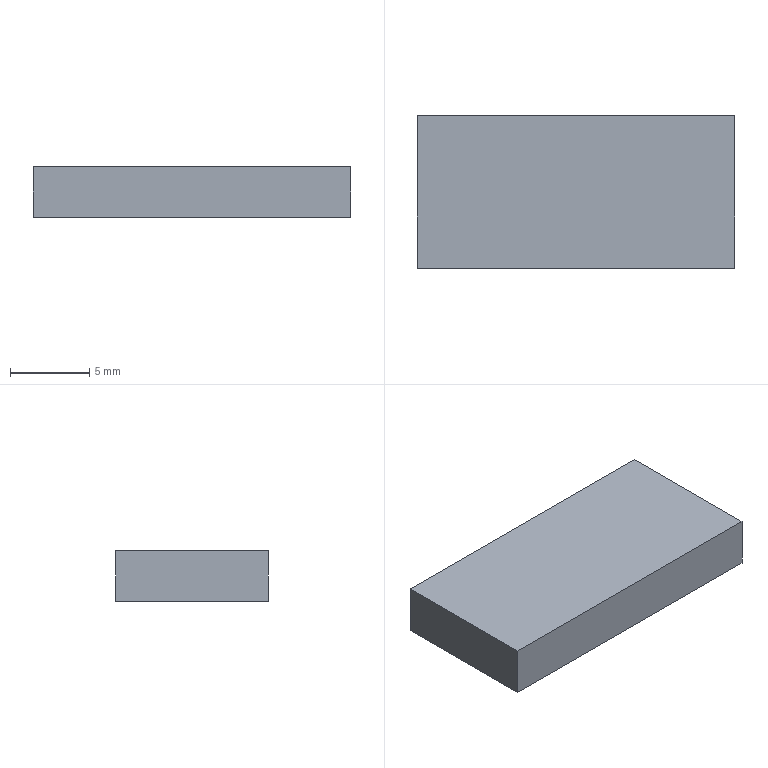Part | SolidWorks | features FlatPattern 1, SMBaseFlange 1, SheetMetal 1 | 1 solid | 6 faces | box 20 x 9.6 x 3.2 mm | volume 614.4 mm3 | plane 6
STEP:
#1=CARTESIAN_POINT('',(25.558,-133.501,0.));
#2=VERTEX_POINT('',#1);
#3=CARTESIAN_POINT('',(25.558,-123.901,0.));
#4=VERTEX_POINT('',#3);
#5=CARTESIAN_POINT('',(25.558,-123.901,0.));
#6=DIRECTION('',(0.,1.,0.));
#7=VECTOR('',#6,1000.);
#8=LINE('',#5,#7);
#9=EDGE_CURVE('',#2,#4,#8,.T.);
#10=ORIENTED_EDGE('',*,*,#9,.F.);
#11=CARTESIAN_POINT('',(25.558,-133.501,-3.2));
#12=VERTEX_POINT('',#11);
#13=CARTESIAN_POINT('',(25.558,-133.501,-3.2));
#14=DIRECTION('',(0.,0.,1.));
#15=VECTOR('',#14,1000.);
#16=LINE('',#13,#15);
#17=EDGE_CURVE('',#12,#2,#16,.T.);
#18=ORIENTED_EDGE('',*,*,#17,.F.);
#19=CARTESIAN_POINT('',(25.558,-123.901,-3.2));
#20=VERTEX_POINT('',#19);
#21=CARTESIAN_POINT('',(25.558,-123.901,-3.2));
#22=DIRECTION('',(0.,1.,0.));
#23=VECTOR('',#22,1000.);
#24=LINE('',#21,#23);
#25=EDGE_CURVE('',#12,#20,#24,.T.);
#26=ORIENTED_EDGE('',*,*,#25,.T.);
#27=CARTESIAN_POINT('',(25.558,-123.901,-3.2));
#28=DIRECTION('',(0.,0.,1.));
#29=VECTOR('',#28,1000.);
#30=LINE('',#27,#29);
#31=EDGE_CURVE('',#20,#4,#30,.T.);
#32=ORIENTED_EDGE('',*,*,#31,.T.);
#33=EDGE_LOOP('',(#10,#18,#26,#32));
#34=FACE_OUTER_BOUND('',#33,.T.);
#35=CARTESIAN_POINT('',(25.558,-123.901,-3.2));
#36=DIRECTION('',(1.,0.,0.));
#37=DIRECTION('',(0.,0.,-1.));
#38=AXIS2_PLACEMENT_3D('',#35,#36,#37);
#39=PLANE('',#38);
#40=ADVANCED_FACE('',(#34),#39,.T.);
#41=CARTESIAN_POINT('',(5.558,-133.501,0.));
#42=VERTEX_POINT('',#41);
#43=CARTESIAN_POINT('',(25.558,-133.501,0.));
#44=DIRECTION('',(1.,0.,0.));
#45=VECTOR('',#44,1000.);
#46=LINE('',#43,#45);
#47=EDGE_CURVE('',#42,#2,#46,.T.);
#48=ORIENTED_EDGE('',*,*,#47,.F.);
#49=CARTESIAN_POINT('',(5.558,-133.501,-3.2));
#50=VERTEX_POINT('',#49);
#51=CARTESIAN_POINT('',(5.558,-133.501,-3.2));
#52=DIRECTION('',(0.,0.,1.));
#53=VECTOR('',#52,1000.);
#54=LINE('',#51,#53);
#55=EDGE_CURVE('',#50,#42,#54,.T.);
#56=ORIENTED_EDGE('',*,*,#55,.F.);
#57=CARTESIAN_POINT('',(25.558,-133.501,-3.2));
#58=DIRECTION('',(1.,0.,0.));
#59=VECTOR('',#58,1000.);
#60=LINE('',#57,#59);
#61=EDGE_CURVE('',#50,#12,#60,.T.);
#62=ORIENTED_EDGE('',*,*,#61,.T.);
#63=ORIENTED_EDGE('',*,*,#17,.T.);
#64=EDGE_LOOP('',(#48,#56,#62,#63));
#65=FACE_OUTER_BOUND('',#64,.T.);
#66=CARTESIAN_POINT('',(25.558,-133.501,-3.2));
#67=DIRECTION('',(0.,-1.,0.));
#68=DIRECTION('',(1.,0.,0.));
#69=AXIS2_PLACEMENT_3D('',#66,#67,#68);
#70=PLANE('',#69);
#71=ADVANCED_FACE('',(#65),#70,.T.);
#72=CARTESIAN_POINT('',(5.558,-123.901,0.));
#73=VERTEX_POINT('',#72);
#74=CARTESIAN_POINT('',(5.558,-123.901,0.));
#75=DIRECTION('',(0.,-1.,0.));
#76=VECTOR('',#75,1000.);
#77=LINE('',#74,#76);
#78=EDGE_CURVE('',#73,#42,#77,.T.);
#79=ORIENTED_EDGE('',*,*,#78,.F.);
#80=CARTESIAN_POINT('',(5.558,-123.901,-3.2));
#81=VERTEX_POINT('',#80);
#82=CARTESIAN_POINT('',(5.558,-123.901,-3.2));
#83=DIRECTION('',(0.,0.,1.));
#84=VECTOR('',#83,1000.);
#85=LINE('',#82,#84);
#86=EDGE_CURVE('',#81,#73,#85,.T.);
#87=ORIENTED_EDGE('',*,*,#86,.F.);
#88=CARTESIAN_POINT('',(5.558,-123.901,-3.2));
#89=DIRECTION('',(0.,-1.,0.));
#90=VECTOR('',#89,1000.);
#91=LINE('',#88,#90);
#92=EDGE_CURVE('',#81,#50,#91,.T.);
#93=ORIENTED_EDGE('',*,*,#92,.T.);
#94=ORIENTED_EDGE('',*,*,#55,.T.);
#95=EDGE_LOOP('',(#79,#87,#93,#94));
#96=FACE_OUTER_BOUND('',#95,.T.);
#97=CARTESIAN_POINT('',(5.558,-123.901,-3.2));
#98=DIRECTION('',(-1.,0.,0.));
#99=DIRECTION('',(0.,0.,1.));
#100=AXIS2_PLACEMENT_3D('',#97,#98,#99);
#101=PLANE('',#100);
#102=ADVANCED_FACE('',(#96),#101,.T.);
#103=CARTESIAN_POINT('',(25.558,-123.901,0.));
#104=DIRECTION('',(-1.,0.,0.));
#105=VECTOR('',#104,1000.);
#106=LINE('',#103,#105);
#107=EDGE_CURVE('',#4,#73,#106,.T.);
#108=ORIENTED_EDGE('',*,*,#107,.F.);
#109=ORIENTED_EDGE('',*,*,#31,.F.);
#110=CARTESIAN_POINT('',(25.558,-123.901,-3.2));
#111=DIRECTION('',(-1.,0.,0.));
#112=VECTOR('',#111,1000.);
#113=LINE('',#110,#112);
#114=EDGE_CURVE('',#20,#81,#113,.T.);
#115=ORIENTED_EDGE('',*,*,#114,.T.);
#116=ORIENTED_EDGE('',*,*,#86,.T.);
#117=EDGE_LOOP('',(#108,#109,#115,#116));
#118=FACE_OUTER_BOUND('',#117,.T.);
#119=CARTESIAN_POINT('',(25.558,-123.901,-3.2));
#120=DIRECTION('',(0.,1.,0.));
#121=DIRECTION('',(0.,0.,1.));
#122=AXIS2_PLACEMENT_3D('',#119,#120,#121);
#123=PLANE('',#122);
#124=ADVANCED_FACE('',(#118),#123,.T.);
#125=ORIENTED_EDGE('',*,*,#25,.F.);
#126=ORIENTED_EDGE('',*,*,#61,.F.);
#127=ORIENTED_EDGE('',*,*,#92,.F.);
#128=ORIENTED_EDGE('',*,*,#114,.F.);
#129=EDGE_LOOP('',(#125,#126,#127,#128));
#130=FACE_OUTER_BOUND('',#129,.T.);
#131=CARTESIAN_POINT('',(0.,0.,-3.2));
#132=DIRECTION('',(0.,0.,-1.));
#133=DIRECTION('',(-1.,0.,0.));
#134=AXIS2_PLACEMENT_3D('',#131,#132,#133);
#135=PLANE('',#134);
#136=ADVANCED_FACE('',(#130),#135,.T.);
#137=ORIENTED_EDGE('',*,*,#9,.T.);
#138=ORIENTED_EDGE('',*,*,#107,.T.);
#139=ORIENTED_EDGE('',*,*,#78,.T.);
#140=ORIENTED_EDGE('',*,*,#47,.T.);
#141=EDGE_LOOP('',(#137,#138,#139,#140));
#142=FACE_OUTER_BOUND('',#141,.T.);
#143=CARTESIAN_POINT('',(0.,0.,0.));
#144=DIRECTION('',(0.,0.,-1.));
#145=DIRECTION('',(-1.,0.,0.));
#146=AXIS2_PLACEMENT_3D('',#143,#144,#145);
#147=PLANE('',#146);
#148=ADVANCED_FACE('',(#142),#147,.F.);
#149=CLOSED_SHELL('',(#40,#71,#102,#124,#136,#148));
#150=MANIFOLD_SOLID_BREP('',#149);
#151=CARTESIAN_POINT('',(0.,0.,0.));
#152=DIRECTION('',(0.,0.,1.));
#153=DIRECTION('',(1.,0.,0.));
#154=AXIS2_PLACEMENT_3D('',#151,#152,#153);
#155=(LENGTH_UNIT()NAMED_UNIT(*)SI_UNIT(.MILLI.,.METRE.));
#156=UNCERTAINTY_MEASURE_WITH_UNIT(LENGTH_MEASURE(0.00001),#155,'','');
#157=(NAMED_UNIT(*)PLANE_ANGLE_UNIT()SI_UNIT($,.RADIAN.));
#158=(NAMED_UNIT(*)SI_UNIT($,.STERADIAN.)SOLID_ANGLE_UNIT());
#159=(GEOMETRIC_REPRESENTATION_CONTEXT(3)GLOBAL_UNCERTAINTY_ASSIGNED_CONTEXT((#156))GLOBAL_UNIT_ASSIGNED_CONTEXT((#155,#157,#158))REPRESENTATION_CONTEXT('',''));
#160=ADVANCED_BREP_SHAPE_REPRESENTATION('',(#150,#154),#159);